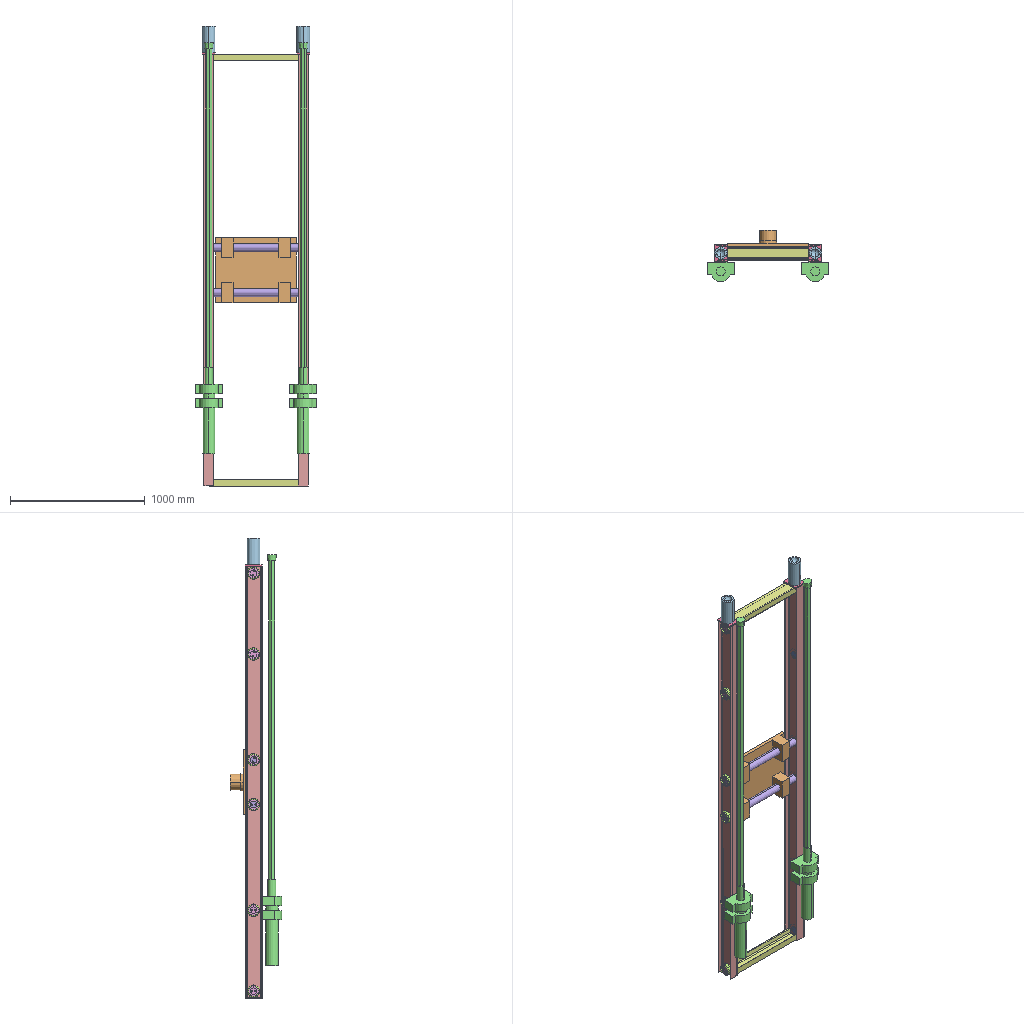Assembly | SolidWorks | 11 different items | 83 placed | box 900 x 380 x 3410 mm
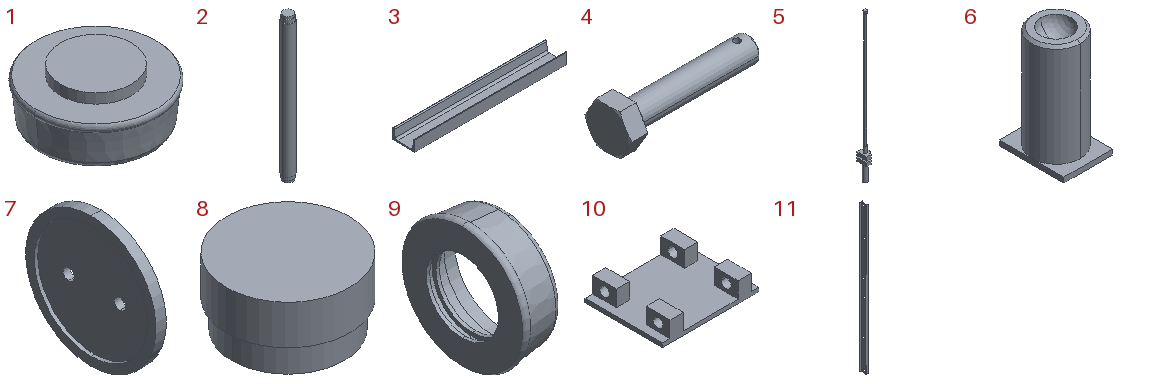Parts list (item | name | quantity | parent item | size | volume | features):
1 | (subassembly) | x12 | - | 94.708 x 94.708 x 39.6 mm | 171130 mm3 | -
2 | - | x2 | - | 60 x 60 x 754.2 mm | 2095819 mm3 | features ICE 4, Extrusion 1
3 | - | x2 | - | 695 x 100 x 48 mm | 885612 mm3 | features Fillet 2, Extrusion 1
4 | - | x24 | in 1 | 34.65 x 11.547 x 10 mm | 1227 mm3 | features RevCut 2, Boss 1, Chamfer 1, Cut 1, Extrusion 1, Fillet 1, LPattern 1, Revolution 1
5 | - | x2 | - | 145 x 200 x 3045 mm | 9881039 mm3 | features ICE 4, Extrusion 1, Revolution 1
6 | - | x2 | - | 95 x 126 x 210 mm | 1477195 mm3 | features Extrusion 1, Revolution 1
7 | - | x12 | in 1 | 6 x 76 x 76 mm | 20111 mm3 | features ICE 1, Revolution 1
8 | - | x12 | in 1 | 55 x 55 x 29.6 mm | 65377 mm3 | features Extrusion 1, ICE 1
9 | - | x12 | in 1 | 32 x 94.708 x 94.708 mm | 83187 mm3 | features Revolution 1
10 | - | x1 | - | 600 x 480 x 222 mm | 11838573 mm3 | features ICE 5, Extrusion 1
11 | - | x2 | - | 74 x 126 x 3200 mm | 4580786 mm3 | features Extrusion 1, ICE 1
Mates (type | each side: item.copy, entity, surface, feature):
In the top assembly
Concentric | 11.1 face cylinder Cut-Extrude1 | 8.1 face cylinder Boss-Extrude2
Concentric | 11.1 face cylinder Cut-Extrude1 | 8.2 face cylinder Boss-Extrude2
Concentric | 11.1 face cylinder Cut-Extrude1 | 8.3 face cylinder Boss-Extrude2
Coincident | 11.1 face plane Boss-Extrude1 | 9.1 face plane Revolve1
Coincident | 11.1 face plane Boss-Extrude1 | 9.2 face plane Revolve1
Coincident | 11.1 face plane Boss-Extrude1 | 9.3 face plane Revolve1
Coincident | 11.1 face plane Boss-Extrude1 | 9.4 face plane Revolve1
Coincident | 11.1 face plane Boss-Extrude1 | 9.5 face plane Revolve1
Coincident | 11.1 face plane Boss-Extrude1 | 9.6 face plane Revolve1
Concentric | 11.1 face cylinder Cut-Extrude1 | 8.4 face cylinder Boss-Extrude2
Coincident | 11.1 face cylinder Cut-Extrude1 | 8.5 edge
Concentric | 11.1 face cylinder Cut-Extrude1 | 8.6 face cylinder Boss-Extrude2
Concentric | 10.1 face cylinder Cut-Extrude1 | 2.1 face cylinder Boss-Extrude3
Concentric | 10.1 face cylinder Cut-Extrude1 | 2.2 face cylinder Boss-Extrude3
Coincident | 2.1 face plane Boss-Extrude2 | 2.2 face plane Boss-Extrude2
Width | 2.1 face plane Boss-Extrude2 | 2.1 face plane Boss-Extrude5 | 10.1 face plane Boss-Extrude2 | 10.1 face plane Boss-Extrude2
Coincident | 11.1 face plane Boss-Extrude1 | 2.2 face plane Boss-Extrude3
Concentric | 9.4 face cone Revolve1 | 2.2 face cylinder Boss-Extrude3
Concentric | 9.1 face cone Revolve1 | 2.1 face cylinder Boss-Extrude3
Coincident | 11.1 face plane Boss-Extrude1 | 5.1 face plane Boss-Extrude5
DistanceDim | 11.1 face plane Boss-Extrude1 | 5.1 face plane Boss-Extrude1
Width | 5.1 face plane Boss-Extrude5 | 5.1 face plane Boss-Extrude5 | 11.1 face plane Boss-Extrude1 | 11.1 face plane Boss-Extrude1
InPlace | 11.2 face plane Boss-Extrude1 | 6.1 plane
Coincident | 11.2 face plane Boss-Extrude1 | 3.1 face plane Base
Coincident | 11.1 face plane Boss-Extrude1 | 3.1 face plane Base
Width | 3.1 face plane Base | 3.1 face plane Base | 11.1 face plane Boss-Extrude1 | 11.1 face plane Boss-Extrude1
Width | 3.2 face plane Base | 3.2 face plane Base | 11.2 face plane Boss-Extrude1 | 11.2 face plane Boss-Extrude1 | 2 times
Coincident | 6.1 face plane Boss-Extrude1 | 3.2 face plane Base
Coincident | 11.1 face plane Boss-Extrude1 | 3.2 face plane Base
In subassembly 1
Concentric | 8.7 face cylinder Boss-Extrude1 | 9.7 face cylinder Revolve1
Concentric | 8.7 face cylinder Boss-Extrude2 | 7.1 face cylinder Revolve1
Concentric | 7.1 face cylinder Cut-Extrude1 | 4.1 face cylinder BaseBody
Coincident | 7.1 face plane Revolve1 | 4.1 face plane Revolve1
Concentric | 7.1 face cylinder Cut-Extrude1 | 4.2 face cylinder BaseBody
Coincident | 7.1 face plane Revolve1 | 4.2 face plane Revolve1